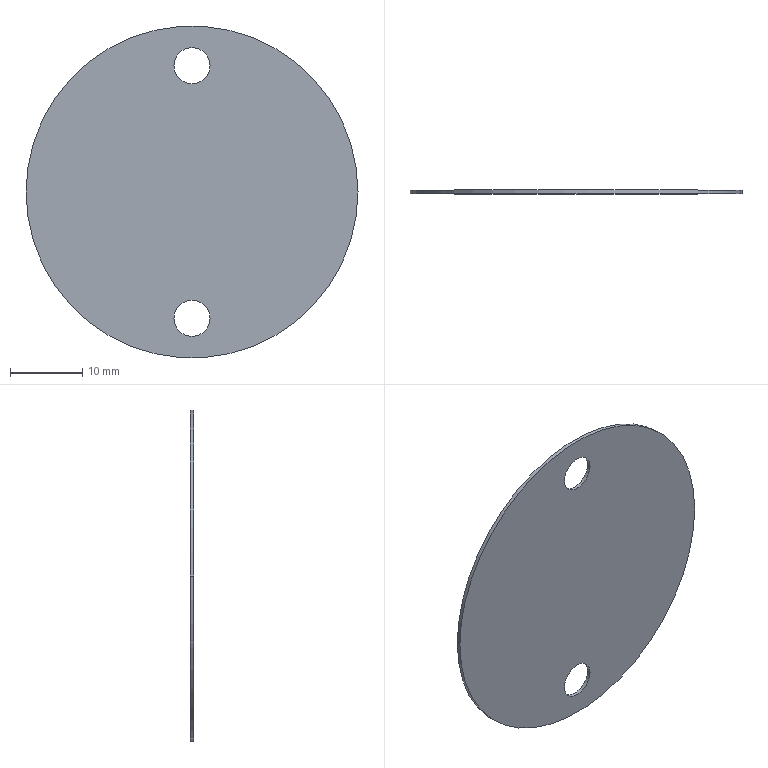Part | STEP file | 1 solid | 8 faces | box 46 x 0.5 x 46 mm | volume 811.316 mm3 | cylinder 6 | plane 2 | commonest cylinder face diameters 5 x4 46 x2
STEP:
#1=CARTESIAN_POINT('',(0.,0.,0.));
#2=DIRECTION('',(0.,0.,1.));
#3=DIRECTION('',(1.,0.,0.));
#4=AXIS2_PLACEMENT_3D('',#1,#2,#3);
#5=CARTESIAN_POINT('',(-2.5,-96.5,17.5));
#6=VERTEX_POINT('',#5);
#7=CARTESIAN_POINT('',(-2.5,-96.,17.5));
#8=VERTEX_POINT('',#7);
#9=CARTESIAN_POINT('',(-2.5,-96.5,17.5));
#10=DIRECTION('',(0.,1.,0.));
#11=VECTOR('',#10,1.);
#12=LINE('',#9,#11);
#13=CARTESIAN_POINT('',(0.,-96.5,17.5));
#14=DIRECTION('',(0.,1.,0.));
#15=DIRECTION('',(-1.,0.,0.));
#16=AXIS2_PLACEMENT_3D('',#13,#14,#15);
#17=CYLINDRICAL_SURFACE('',#16,2.5);
#18=CARTESIAN_POINT('',(6.283,0.));
#19=DIRECTION('',(0.,1.));
#20=VECTOR('',#19,1.);
#21=LINE('',#18,#20);
#22=(GEOMETRIC_REPRESENTATION_CONTEXT(2)PARAMETRIC_REPRESENTATION_CONTEXT()REPRESENTATION_CONTEXT('',''));
#23=DEFINITIONAL_REPRESENTATION('',(#21),#22);
#24=PCURVE('',#17,#23);
#25=CARTESIAN_POINT('',(0.,-96.5,17.5));
#26=DIRECTION('',(0.,1.,0.));
#27=DIRECTION('',(-1.,0.,0.));
#28=AXIS2_PLACEMENT_3D('',#25,#26,#27);
#29=CYLINDRICAL_SURFACE('',#28,2.5);
#30=CARTESIAN_POINT('',(0.,0.));
#31=DIRECTION('',(0.,1.));
#32=VECTOR('',#31,1.);
#33=LINE('',#30,#32);
#34=(GEOMETRIC_REPRESENTATION_CONTEXT(2)PARAMETRIC_REPRESENTATION_CONTEXT()REPRESENTATION_CONTEXT('',''));
#35=DEFINITIONAL_REPRESENTATION('',(#33),#34);
#36=PCURVE('',#29,#35);
#37=SURFACE_CURVE('',#12,(#24,#36),.PCURVE_S1.);
#38=EDGE_CURVE('',#6,#8,#37,.T.);
#39=ORIENTED_EDGE('',*,*,#38,.T.);
#40=CARTESIAN_POINT('',(2.5,-96.,17.5));
#41=VERTEX_POINT('',#40);
#42=CARTESIAN_POINT('',(0.,-96.,17.5));
#43=DIRECTION('',(0.,1.,0.));
#44=DIRECTION('',(-1.,0.,0.));
#45=AXIS2_PLACEMENT_3D('',#42,#43,#44);
#46=CIRCLE('',#45,2.5);
#47=CARTESIAN_POINT('',(0.,0.5));
#48=DIRECTION('',(1.,0.));
#49=VECTOR('',#48,1.);
#50=LINE('',#47,#49);
#51=(GEOMETRIC_REPRESENTATION_CONTEXT(2)PARAMETRIC_REPRESENTATION_CONTEXT()REPRESENTATION_CONTEXT('',''));
#52=DEFINITIONAL_REPRESENTATION('',(#50),#51);
#53=PCURVE('',#17,#52);
#54=CARTESIAN_POINT('',(23.92,-96.,23.92));
#55=DIRECTION('',(0.,1.,0.));
#56=DIRECTION('',(0.,0.,-1.));
#57=AXIS2_PLACEMENT_3D('',#54,#55,#56);
#58=PLANE('',#57);
#59=CARTESIAN_POINT('',(6.42,23.92));
#60=DIRECTION('',(0.,1.));
#61=AXIS2_PLACEMENT_2D('',#59,#60);
#62=CIRCLE('',#61,2.5);
#63=(GEOMETRIC_REPRESENTATION_CONTEXT(2)PARAMETRIC_REPRESENTATION_CONTEXT()REPRESENTATION_CONTEXT('',''));
#64=DEFINITIONAL_REPRESENTATION('',(#62),#63);
#65=PCURVE('',#58,#64);
#66=SURFACE_CURVE('',#46,(#53,#65),.PCURVE_S1.);
#67=EDGE_CURVE('',#41,#8,#66,.T.);
#68=ORIENTED_EDGE('',*,*,#67,.F.);
#69=CARTESIAN_POINT('',(2.5,-96.5,17.5));
#70=VERTEX_POINT('',#69);
#71=CARTESIAN_POINT('',(2.5,-96.5,17.5));
#72=DIRECTION('',(0.,1.,0.));
#73=VECTOR('',#72,1.);
#74=LINE('',#71,#73);
#75=CARTESIAN_POINT('',(3.142,0.));
#76=DIRECTION('',(0.,1.));
#77=VECTOR('',#76,1.);
#78=LINE('',#75,#77);
#79=(GEOMETRIC_REPRESENTATION_CONTEXT(2)PARAMETRIC_REPRESENTATION_CONTEXT()REPRESENTATION_CONTEXT('',''));
#80=DEFINITIONAL_REPRESENTATION('',(#78),#79);
#81=PCURVE('',#17,#80);
#82=CARTESIAN_POINT('',(3.142,0.));
#83=DIRECTION('',(0.,1.));
#84=VECTOR('',#83,1.);
#85=LINE('',#82,#84);
#86=(GEOMETRIC_REPRESENTATION_CONTEXT(2)PARAMETRIC_REPRESENTATION_CONTEXT()REPRESENTATION_CONTEXT('',''));
#87=DEFINITIONAL_REPRESENTATION('',(#85),#86);
#88=PCURVE('',#29,#87);
#89=SURFACE_CURVE('',#74,(#81,#88),.PCURVE_S1.);
#90=EDGE_CURVE('',#70,#41,#89,.T.);
#91=ORIENTED_EDGE('',*,*,#90,.F.);
#92=CARTESIAN_POINT('',(0.,-96.5,17.5));
#93=DIRECTION('',(0.,-1.,0.));
#94=DIRECTION('',(-1.,0.,0.));
#95=AXIS2_PLACEMENT_3D('',#92,#93,#94);
#96=CIRCLE('',#95,2.5);
#97=CARTESIAN_POINT('',(6.283,0.));
#98=DIRECTION('',(-1.,0.));
#99=VECTOR('',#98,1.);
#100=LINE('',#97,#99);
#101=(GEOMETRIC_REPRESENTATION_CONTEXT(2)PARAMETRIC_REPRESENTATION_CONTEXT()REPRESENTATION_CONTEXT('',''));
#102=DEFINITIONAL_REPRESENTATION('',(#100),#101);
#103=PCURVE('',#17,#102);
#104=CARTESIAN_POINT('',(23.92,-96.5,23.92));
#105=DIRECTION('',(0.,1.,0.));
#106=DIRECTION('',(0.,0.,-1.));
#107=AXIS2_PLACEMENT_3D('',#104,#105,#106);
#108=PLANE('',#107);
#109=CARTESIAN_POINT('',(6.42,26.42));
#110=CARTESIAN_POINT('',(10.75,26.42));
#111=CARTESIAN_POINT('',(8.585,22.67));
#112=CARTESIAN_POINT('',(6.42,18.92));
#113=CARTESIAN_POINT('',(4.255,22.67));
#114=CARTESIAN_POINT('',(2.09,26.42));
#115=CARTESIAN_POINT('',(6.42,26.42));
#116=(BOUNDED_CURVE()B_SPLINE_CURVE(2,(#109,#110,#111,#112,#113,#114,#115),.UNSPECIFIED.,.T.,.F.)B_SPLINE_CURVE_WITH_KNOTS((1,2,2,2,2,1),(-2.094,0.,2.094,4.189,6.283,8.378),.UNSPECIFIED.)CURVE()GEOMETRIC_REPRESENTATION_ITEM()RATIONAL_B_SPLINE_CURVE((1.,0.5,1.,0.5,1.,0.5,1.))REPRESENTATION_ITEM(''));
#117=(GEOMETRIC_REPRESENTATION_CONTEXT(2)PARAMETRIC_REPRESENTATION_CONTEXT()REPRESENTATION_CONTEXT('',''));
#118=DEFINITIONAL_REPRESENTATION('',(#116),#117);
#119=PCURVE('',#108,#118);
#120=SURFACE_CURVE('',#96,(#103,#119),.PCURVE_S1.);
#121=EDGE_CURVE('',#6,#70,#120,.T.);
#122=ORIENTED_EDGE('',*,*,#121,.F.);
#123=EDGE_LOOP('',(#39,#68,#91,#122));
#124=FACE_BOUND('',#123,.F.);
#125=ADVANCED_FACE('',(#124),#17,.F.);
#126=CARTESIAN_POINT('',(-2.5,-96.5,-17.5));
#127=VERTEX_POINT('',#126);
#128=CARTESIAN_POINT('',(-2.5,-96.,-17.5));
#129=VERTEX_POINT('',#128);
#130=CARTESIAN_POINT('',(-2.5,-96.5,-17.5));
#131=DIRECTION('',(0.,1.,0.));
#132=VECTOR('',#131,1.);
#133=LINE('',#130,#132);
#134=CARTESIAN_POINT('',(0.,-96.5,-17.5));
#135=DIRECTION('',(0.,1.,0.));
#136=DIRECTION('',(-1.,0.,0.));
#137=AXIS2_PLACEMENT_3D('',#134,#135,#136);
#138=CYLINDRICAL_SURFACE('',#137,2.5);
#139=CARTESIAN_POINT('',(6.283,0.));
#140=DIRECTION('',(0.,1.));
#141=VECTOR('',#140,1.);
#142=LINE('',#139,#141);
#143=(GEOMETRIC_REPRESENTATION_CONTEXT(2)PARAMETRIC_REPRESENTATION_CONTEXT()REPRESENTATION_CONTEXT('',''));
#144=DEFINITIONAL_REPRESENTATION('',(#142),#143);
#145=PCURVE('',#138,#144);
#146=CARTESIAN_POINT('',(0.,-96.5,-17.5));
#147=DIRECTION('',(0.,1.,0.));
#148=DIRECTION('',(-1.,0.,0.));
#149=AXIS2_PLACEMENT_3D('',#146,#147,#148);
#150=CYLINDRICAL_SURFACE('',#149,2.5);
#151=CARTESIAN_POINT('',(0.,0.));
#152=DIRECTION('',(0.,1.));
#153=VECTOR('',#152,1.);
#154=LINE('',#151,#153);
#155=(GEOMETRIC_REPRESENTATION_CONTEXT(2)PARAMETRIC_REPRESENTATION_CONTEXT()REPRESENTATION_CONTEXT('',''));
#156=DEFINITIONAL_REPRESENTATION('',(#154),#155);
#157=PCURVE('',#150,#156);
#158=SURFACE_CURVE('',#133,(#145,#157),.PCURVE_S1.);
#159=EDGE_CURVE('',#127,#129,#158,.T.);
#160=ORIENTED_EDGE('',*,*,#159,.T.);
#161=CARTESIAN_POINT('',(2.5,-96.,-17.5));
#162=VERTEX_POINT('',#161);
#163=CARTESIAN_POINT('',(0.,-96.,-17.5));
#164=DIRECTION('',(0.,1.,0.));
#165=DIRECTION('',(-1.,0.,0.));
#166=AXIS2_PLACEMENT_3D('',#163,#164,#165);
#167=CIRCLE('',#166,2.5);
#168=CARTESIAN_POINT('',(0.,0.5));
#169=DIRECTION('',(1.,0.));
#170=VECTOR('',#169,1.);
#171=LINE('',#168,#170);
#172=(GEOMETRIC_REPRESENTATION_CONTEXT(2)PARAMETRIC_REPRESENTATION_CONTEXT()REPRESENTATION_CONTEXT('',''));
#173=DEFINITIONAL_REPRESENTATION('',(#171),#172);
#174=PCURVE('',#138,#173);
#175=CARTESIAN_POINT('',(41.42,23.92));
#176=DIRECTION('',(0.,1.));
#177=AXIS2_PLACEMENT_2D('',#175,#176);
#178=CIRCLE('',#177,2.5);
#179=(GEOMETRIC_REPRESENTATION_CONTEXT(2)PARAMETRIC_REPRESENTATION_CONTEXT()REPRESENTATION_CONTEXT('',''));
#180=DEFINITIONAL_REPRESENTATION('',(#178),#179);
#181=PCURVE('',#58,#180);
#182=SURFACE_CURVE('',#167,(#174,#181),.PCURVE_S1.);
#183=EDGE_CURVE('',#162,#129,#182,.T.);
#184=ORIENTED_EDGE('',*,*,#183,.F.);
#185=CARTESIAN_POINT('',(2.5,-96.5,-17.5));
#186=VERTEX_POINT('',#185);
#187=CARTESIAN_POINT('',(2.5,-96.5,-17.5));
#188=DIRECTION('',(0.,1.,0.));
#189=VECTOR('',#188,1.);
#190=LINE('',#187,#189);
#191=CARTESIAN_POINT('',(3.142,0.));
#192=DIRECTION('',(0.,1.));
#193=VECTOR('',#192,1.);
#194=LINE('',#191,#193);
#195=(GEOMETRIC_REPRESENTATION_CONTEXT(2)PARAMETRIC_REPRESENTATION_CONTEXT()REPRESENTATION_CONTEXT('',''));
#196=DEFINITIONAL_REPRESENTATION('',(#194),#195);
#197=PCURVE('',#138,#196);
#198=CARTESIAN_POINT('',(3.142,0.));
#199=DIRECTION('',(0.,1.));
#200=VECTOR('',#199,1.);
#201=LINE('',#198,#200);
#202=(GEOMETRIC_REPRESENTATION_CONTEXT(2)PARAMETRIC_REPRESENTATION_CONTEXT()REPRESENTATION_CONTEXT('',''));
#203=DEFINITIONAL_REPRESENTATION('',(#201),#202);
#204=PCURVE('',#150,#203);
#205=SURFACE_CURVE('',#190,(#197,#204),.PCURVE_S1.);
#206=EDGE_CURVE('',#186,#162,#205,.T.);
#207=ORIENTED_EDGE('',*,*,#206,.F.);
#208=CARTESIAN_POINT('',(0.,-96.5,-17.5));
#209=DIRECTION('',(0.,-1.,0.));
#210=DIRECTION('',(-1.,0.,0.));
#211=AXIS2_PLACEMENT_3D('',#208,#209,#210);
#212=CIRCLE('',#211,2.5);
#213=CARTESIAN_POINT('',(6.283,0.));
#214=DIRECTION('',(-1.,0.));
#215=VECTOR('',#214,1.);
#216=LINE('',#213,#215);
#217=(GEOMETRIC_REPRESENTATION_CONTEXT(2)PARAMETRIC_REPRESENTATION_CONTEXT()REPRESENTATION_CONTEXT('',''));
#218=DEFINITIONAL_REPRESENTATION('',(#216),#217);
#219=PCURVE('',#138,#218);
#220=CARTESIAN_POINT('',(41.42,26.42));
#221=CARTESIAN_POINT('',(45.75,26.42));
#222=CARTESIAN_POINT('',(43.585,22.67));
#223=CARTESIAN_POINT('',(41.42,18.92));
#224=CARTESIAN_POINT('',(39.255,22.67));
#225=CARTESIAN_POINT('',(37.09,26.42));
#226=CARTESIAN_POINT('',(41.42,26.42));
#227=(BOUNDED_CURVE()B_SPLINE_CURVE(2,(#220,#221,#222,#223,#224,#225,#226),.UNSPECIFIED.,.T.,.F.)B_SPLINE_CURVE_WITH_KNOTS((1,2,2,2,2,1),(-2.094,0.,2.094,4.189,6.283,8.378),.UNSPECIFIED.)CURVE()GEOMETRIC_REPRESENTATION_ITEM()RATIONAL_B_SPLINE_CURVE((1.,0.5,1.,0.5,1.,0.5,1.))REPRESENTATION_ITEM(''));
#228=(GEOMETRIC_REPRESENTATION_CONTEXT(2)PARAMETRIC_REPRESENTATION_CONTEXT()REPRESENTATION_CONTEXT('',''));
#229=DEFINITIONAL_REPRESENTATION('',(#227),#228);
#230=PCURVE('',#108,#229);
#231=SURFACE_CURVE('',#212,(#219,#230),.PCURVE_S1.);
#232=EDGE_CURVE('',#127,#186,#231,.T.);
#233=ORIENTED_EDGE('',*,*,#232,.F.);
#234=EDGE_LOOP('',(#160,#184,#207,#233));
#235=FACE_BOUND('',#234,.F.);
#236=ADVANCED_FACE('',(#235),#138,.F.);
#237=CARTESIAN_POINT('',(-23.,-96.5,0.));
#238=VERTEX_POINT('',#237);
#239=CARTESIAN_POINT('',(23.,-96.5,0.));
#240=VERTEX_POINT('',#239);
#241=CARTESIAN_POINT('',(0.,-96.5,0.));
#242=DIRECTION('',(0.,1.,0.));
#243=DIRECTION('',(-1.,0.,0.));
#244=AXIS2_PLACEMENT_3D('',#241,#242,#243);
#245=CIRCLE('',#244,23.);
#246=CARTESIAN_POINT('',(0.,-96.5,0.));
#247=DIRECTION('',(0.,1.,0.));
#248=DIRECTION('',(-1.,0.,0.));
#249=AXIS2_PLACEMENT_3D('',#246,#247,#248);
#250=CYLINDRICAL_SURFACE('',#249,23.);
#251=CARTESIAN_POINT('',(0.,0.));
#252=DIRECTION('',(1.,0.));
#253=VECTOR('',#252,1.);
#254=LINE('',#251,#253);
#255=(GEOMETRIC_REPRESENTATION_CONTEXT(2)PARAMETRIC_REPRESENTATION_CONTEXT()REPRESENTATION_CONTEXT('',''));
#256=DEFINITIONAL_REPRESENTATION('',(#254),#255);
#257=PCURVE('',#250,#256);
#258=CARTESIAN_POINT('',(23.92,23.92));
#259=DIRECTION('',(0.,1.));
#260=AXIS2_PLACEMENT_2D('',#258,#259);
#261=CIRCLE('',#260,23.);
#262=(GEOMETRIC_REPRESENTATION_CONTEXT(2)PARAMETRIC_REPRESENTATION_CONTEXT()REPRESENTATION_CONTEXT('',''));
#263=DEFINITIONAL_REPRESENTATION('',(#261),#262);
#264=PCURVE('',#108,#263);
#265=SURFACE_CURVE('',#245,(#257,#264),.PCURVE_S1.);
#266=EDGE_CURVE('',#238,#240,#265,.T.);
#267=ORIENTED_EDGE('',*,*,#266,.T.);
#268=CARTESIAN_POINT('',(23.,-96.,0.));
#269=VERTEX_POINT('',#268);
#270=CARTESIAN_POINT('',(23.,-96.5,0.));
#271=DIRECTION('',(0.,1.,0.));
#272=VECTOR('',#271,1.);
#273=LINE('',#270,#272);
#274=CARTESIAN_POINT('',(3.142,0.));
#275=DIRECTION('',(0.,1.));
#276=VECTOR('',#275,1.);
#277=LINE('',#274,#276);
#278=(GEOMETRIC_REPRESENTATION_CONTEXT(2)PARAMETRIC_REPRESENTATION_CONTEXT()REPRESENTATION_CONTEXT('',''));
#279=DEFINITIONAL_REPRESENTATION('',(#277),#278);
#280=PCURVE('',#250,#279);
#281=CARTESIAN_POINT('',(0.,-96.5,0.));
#282=DIRECTION('',(0.,1.,0.));
#283=DIRECTION('',(-1.,0.,0.));
#284=AXIS2_PLACEMENT_3D('',#281,#282,#283);
#285=CYLINDRICAL_SURFACE('',#284,23.);
#286=CARTESIAN_POINT('',(3.142,0.));
#287=DIRECTION('',(0.,1.));
#288=VECTOR('',#287,1.);
#289=LINE('',#286,#288);
#290=(GEOMETRIC_REPRESENTATION_CONTEXT(2)PARAMETRIC_REPRESENTATION_CONTEXT()REPRESENTATION_CONTEXT('',''));
#291=DEFINITIONAL_REPRESENTATION('',(#289),#290);
#292=PCURVE('',#285,#291);
#293=SURFACE_CURVE('',#273,(#280,#292),.PCURVE_S1.);
#294=EDGE_CURVE('',#240,#269,#293,.T.);
#295=ORIENTED_EDGE('',*,*,#294,.T.);
#296=CARTESIAN_POINT('',(-23.,-96.,0.));
#297=VERTEX_POINT('',#296);
#298=CARTESIAN_POINT('',(0.,-96.,0.));
#299=DIRECTION('',(0.,1.,0.));
#300=DIRECTION('',(-1.,0.,0.));
#301=AXIS2_PLACEMENT_3D('',#298,#299,#300);
#302=CIRCLE('',#301,23.);
#303=CARTESIAN_POINT('',(0.,0.5));
#304=DIRECTION('',(1.,0.));
#305=VECTOR('',#304,1.);
#306=LINE('',#303,#305);
#307=(GEOMETRIC_REPRESENTATION_CONTEXT(2)PARAMETRIC_REPRESENTATION_CONTEXT()REPRESENTATION_CONTEXT('',''));
#308=DEFINITIONAL_REPRESENTATION('',(#306),#307);
#309=PCURVE('',#250,#308);
#310=CARTESIAN_POINT('',(23.92,23.92));
#311=DIRECTION('',(0.,1.));
#312=AXIS2_PLACEMENT_2D('',#310,#311);
#313=CIRCLE('',#312,23.);
#314=(GEOMETRIC_REPRESENTATION_CONTEXT(2)PARAMETRIC_REPRESENTATION_CONTEXT()REPRESENTATION_CONTEXT('',''));
#315=DEFINITIONAL_REPRESENTATION('',(#313),#314);
#316=PCURVE('',#58,#315);
#317=SURFACE_CURVE('',#302,(#309,#316),.PCURVE_S1.);
#318=EDGE_CURVE('',#297,#269,#317,.T.);
#319=ORIENTED_EDGE('',*,*,#318,.F.);
#320=CARTESIAN_POINT('',(-23.,-96.5,0.));
#321=DIRECTION('',(0.,1.,0.));
#322=VECTOR('',#321,1.);
#323=LINE('',#320,#322);
#324=CARTESIAN_POINT('',(0.,0.));
#325=DIRECTION('',(0.,1.));
#326=VECTOR('',#325,1.);
#327=LINE('',#324,#326);
#328=(GEOMETRIC_REPRESENTATION_CONTEXT(2)PARAMETRIC_REPRESENTATION_CONTEXT()REPRESENTATION_CONTEXT('',''));
#329=DEFINITIONAL_REPRESENTATION('',(#327),#328);
#330=PCURVE('',#250,#329);
#331=CARTESIAN_POINT('',(6.283,0.));
#332=DIRECTION('',(0.,1.));
#333=VECTOR('',#332,1.);
#334=LINE('',#331,#333);
#335=(GEOMETRIC_REPRESENTATION_CONTEXT(2)PARAMETRIC_REPRESENTATION_CONTEXT()REPRESENTATION_CONTEXT('',''));
#336=DEFINITIONAL_REPRESENTATION('',(#334),#335);
#337=PCURVE('',#285,#336);
#338=SURFACE_CURVE('',#323,(#330,#337),.PCURVE_S1.);
#339=EDGE_CURVE('',#238,#297,#338,.T.);
#340=ORIENTED_EDGE('',*,*,#339,.F.);
#341=EDGE_LOOP('',(#267,#295,#319,#340));
#342=FACE_BOUND('',#341,.T.);
#343=ADVANCED_FACE('',(#342),#250,.T.);
#344=CARTESIAN_POINT('',(0.,-96.,17.5));
#345=DIRECTION('',(0.,1.,0.));
#346=DIRECTION('',(-1.,0.,0.));
#347=AXIS2_PLACEMENT_3D('',#344,#345,#346);
#348=CIRCLE('',#347,2.5);
#349=CARTESIAN_POINT('',(6.42,23.92));
#350=DIRECTION('',(0.,1.));
#351=AXIS2_PLACEMENT_2D('',#349,#350);
#352=CIRCLE('',#351,2.5);
#353=(GEOMETRIC_REPRESENTATION_CONTEXT(2)PARAMETRIC_REPRESENTATION_CONTEXT()REPRESENTATION_CONTEXT('',''));
#354=DEFINITIONAL_REPRESENTATION('',(#352),#353);
#355=PCURVE('',#58,#354);
#356=CARTESIAN_POINT('',(0.,0.5));
#357=DIRECTION('',(1.,0.));
#358=VECTOR('',#357,1.);
#359=LINE('',#356,#358);
#360=(GEOMETRIC_REPRESENTATION_CONTEXT(2)PARAMETRIC_REPRESENTATION_CONTEXT()REPRESENTATION_CONTEXT('',''));
#361=DEFINITIONAL_REPRESENTATION('',(#359),#360);
#362=PCURVE('',#29,#361);
#363=SURFACE_CURVE('',#348,(#355,#362),.PCURVE_S1.);
#364=EDGE_CURVE('',#8,#41,#363,.T.);
#365=ORIENTED_EDGE('',*,*,#364,.F.);
#366=ORIENTED_EDGE('',*,*,#67,.F.);
#367=EDGE_LOOP('',(#365,#366));
#368=FACE_BOUND('',#367,.T.);
#369=CARTESIAN_POINT('',(0.,-96.,-17.5));
#370=DIRECTION('',(0.,1.,0.));
#371=DIRECTION('',(-1.,0.,0.));
#372=AXIS2_PLACEMENT_3D('',#369,#370,#371);
#373=CIRCLE('',#372,2.5);
#374=CARTESIAN_POINT('',(41.42,23.92));
#375=DIRECTION('',(0.,1.));
#376=AXIS2_PLACEMENT_2D('',#374,#375);
#377=CIRCLE('',#376,2.5);
#378=(GEOMETRIC_REPRESENTATION_CONTEXT(2)PARAMETRIC_REPRESENTATION_CONTEXT()REPRESENTATION_CONTEXT('',''));
#379=DEFINITIONAL_REPRESENTATION('',(#377),#378);
#380=PCURVE('',#58,#379);
#381=CARTESIAN_POINT('',(0.,0.5));
#382=DIRECTION('',(1.,0.));
#383=VECTOR('',#382,1.);
#384=LINE('',#381,#383);
#385=(GEOMETRIC_REPRESENTATION_CONTEXT(2)PARAMETRIC_REPRESENTATION_CONTEXT()REPRESENTATION_CONTEXT('',''));
#386=DEFINITIONAL_REPRESENTATION('',(#384),#385);
#387=PCURVE('',#150,#386);
#388=SURFACE_CURVE('',#373,(#380,#387),.PCURVE_S1.);
#389=EDGE_CURVE('',#129,#162,#388,.T.);
#390=ORIENTED_EDGE('',*,*,#389,.F.);
#391=ORIENTED_EDGE('',*,*,#183,.F.);
#392=EDGE_LOOP('',(#390,#391));
#393=FACE_BOUND('',#392,.T.);
#394=ORIENTED_EDGE('',*,*,#318,.T.);
#395=CARTESIAN_POINT('',(0.,-96.,0.));
#396=DIRECTION('',(0.,1.,0.));
#397=DIRECTION('',(-1.,0.,0.));
#398=AXIS2_PLACEMENT_3D('',#395,#396,#397);
#399=CIRCLE('',#398,23.);
#400=CARTESIAN_POINT('',(23.92,23.92));
#401=DIRECTION('',(0.,1.));
#402=AXIS2_PLACEMENT_2D('',#400,#401);
#403=CIRCLE('',#402,23.);
#404=(GEOMETRIC_REPRESENTATION_CONTEXT(2)PARAMETRIC_REPRESENTATION_CONTEXT()REPRESENTATION_CONTEXT('',''));
#405=DEFINITIONAL_REPRESENTATION('',(#403),#404);
#406=PCURVE('',#58,#405);
#407=CARTESIAN_POINT('',(0.,0.5));
#408=DIRECTION('',(1.,0.));
#409=VECTOR('',#408,1.);
#410=LINE('',#407,#409);
#411=(GEOMETRIC_REPRESENTATION_CONTEXT(2)PARAMETRIC_REPRESENTATION_CONTEXT()REPRESENTATION_CONTEXT('',''));
#412=DEFINITIONAL_REPRESENTATION('',(#410),#411);
#413=PCURVE('',#285,#412);
#414=SURFACE_CURVE('',#399,(#406,#413),.PCURVE_S1.);
#415=EDGE_CURVE('',#269,#297,#414,.T.);
#416=ORIENTED_EDGE('',*,*,#415,.T.);
#417=EDGE_LOOP('',(#394,#416));
#418=FACE_BOUND('',#417,.T.);
#419=ADVANCED_FACE('',(#368,#393,#418),#58,.T.);
#420=ORIENTED_EDGE('',*,*,#294,.F.);
#421=CARTESIAN_POINT('',(0.,-96.5,0.));
#422=DIRECTION('',(0.,1.,0.));
#423=DIRECTION('',(-1.,0.,0.));
#424=AXIS2_PLACEMENT_3D('',#421,#422,#423);
#425=CIRCLE('',#424,23.);
#426=CARTESIAN_POINT('',(0.,0.));
#427=DIRECTION('',(1.,0.));
#428=VECTOR('',#427,1.);
#429=LINE('',#426,#428);
#430=(GEOMETRIC_REPRESENTATION_CONTEXT(2)PARAMETRIC_REPRESENTATION_CONTEXT()REPRESENTATION_CONTEXT('',''));
#431=DEFINITIONAL_REPRESENTATION('',(#429),#430);
#432=PCURVE('',#285,#431);
#433=CARTESIAN_POINT('',(23.92,23.92));
#434=DIRECTION('',(0.,1.));
#435=AXIS2_PLACEMENT_2D('',#433,#434);
#436=CIRCLE('',#435,23.);
#437=(GEOMETRIC_REPRESENTATION_CONTEXT(2)PARAMETRIC_REPRESENTATION_CONTEXT()REPRESENTATION_CONTEXT('',''));
#438=DEFINITIONAL_REPRESENTATION('',(#436),#437);
#439=PCURVE('',#108,#438);
#440=SURFACE_CURVE('',#425,(#432,#439),.PCURVE_S1.);
#441=EDGE_CURVE('',#240,#238,#440,.T.);
#442=ORIENTED_EDGE('',*,*,#441,.T.);
#443=ORIENTED_EDGE('',*,*,#339,.T.);
#444=ORIENTED_EDGE('',*,*,#415,.F.);
#445=EDGE_LOOP('',(#420,#442,#443,#444));
#446=FACE_BOUND('',#445,.T.);
#447=ADVANCED_FACE('',(#446),#285,.T.);
#448=ORIENTED_EDGE('',*,*,#389,.F.);
#449=ORIENTED_EDGE('',*,*,#159,.F.);
#450=CARTESIAN_POINT('',(0.,-96.5,-17.5));
#451=DIRECTION('',(0.,-1.,0.));
#452=DIRECTION('',(-1.,0.,0.));
#453=AXIS2_PLACEMENT_3D('',#450,#451,#452);
#454=CIRCLE('',#453,2.5);
#455=CARTESIAN_POINT('',(6.283,0.));
#456=DIRECTION('',(-1.,0.));
#457=VECTOR('',#456,1.);
#458=LINE('',#455,#457);
#459=(GEOMETRIC_REPRESENTATION_CONTEXT(2)PARAMETRIC_REPRESENTATION_CONTEXT()REPRESENTATION_CONTEXT('',''));
#460=DEFINITIONAL_REPRESENTATION('',(#458),#459);
#461=PCURVE('',#150,#460);
#462=CARTESIAN_POINT('',(41.42,26.42));
#463=CARTESIAN_POINT('',(45.75,26.42));
#464=CARTESIAN_POINT('',(43.585,22.67));
#465=CARTESIAN_POINT('',(41.42,18.92));
#466=CARTESIAN_POINT('',(39.255,22.67));
#467=CARTESIAN_POINT('',(37.09,26.42));
#468=CARTESIAN_POINT('',(41.42,26.42));
#469=(BOUNDED_CURVE()B_SPLINE_CURVE(2,(#462,#463,#464,#465,#466,#467,#468),.UNSPECIFIED.,.T.,.F.)B_SPLINE_CURVE_WITH_KNOTS((1,2,2,2,2,1),(-2.094,0.,2.094,4.189,6.283,8.378),.UNSPECIFIED.)CURVE()GEOMETRIC_REPRESENTATION_ITEM()RATIONAL_B_SPLINE_CURVE((1.,0.5,1.,0.5,1.,0.5,1.))REPRESENTATION_ITEM(''));
#470=(GEOMETRIC_REPRESENTATION_CONTEXT(2)PARAMETRIC_REPRESENTATION_CONTEXT()REPRESENTATION_CONTEXT('',''));
#471=DEFINITIONAL_REPRESENTATION('',(#469),#470);
#472=PCURVE('',#108,#471);
#473=SURFACE_CURVE('',#454,(#461,#472),.PCURVE_S1.);
#474=EDGE_CURVE('',#186,#127,#473,.T.);
#475=ORIENTED_EDGE('',*,*,#474,.F.);
#476=ORIENTED_EDGE('',*,*,#206,.T.);
#477=EDGE_LOOP('',(#448,#449,#475,#476));
#478=FACE_BOUND('',#477,.F.);
#479=ADVANCED_FACE('',(#478),#150,.F.);
#480=ORIENTED_EDGE('',*,*,#364,.F.);
#481=ORIENTED_EDGE('',*,*,#38,.F.);
#482=CARTESIAN_POINT('',(0.,-96.5,17.5));
#483=DIRECTION('',(0.,-1.,0.));
#484=DIRECTION('',(-1.,0.,0.));
#485=AXIS2_PLACEMENT_3D('',#482,#483,#484);
#486=CIRCLE('',#485,2.5);
#487=CARTESIAN_POINT('',(6.283,0.));
#488=DIRECTION('',(-1.,0.));
#489=VECTOR('',#488,1.);
#490=LINE('',#487,#489);
#491=(GEOMETRIC_REPRESENTATION_CONTEXT(2)PARAMETRIC_REPRESENTATION_CONTEXT()REPRESENTATION_CONTEXT('',''));
#492=DEFINITIONAL_REPRESENTATION('',(#490),#491);
#493=PCURVE('',#29,#492);
#494=CARTESIAN_POINT('',(6.42,26.42));
#495=CARTESIAN_POINT('',(10.75,26.42));
#496=CARTESIAN_POINT('',(8.585,22.67));
#497=CARTESIAN_POINT('',(6.42,18.92));
#498=CARTESIAN_POINT('',(4.255,22.67));
#499=CARTESIAN_POINT('',(2.09,26.42));
#500=CARTESIAN_POINT('',(6.42,26.42));
#501=(BOUNDED_CURVE()B_SPLINE_CURVE(2,(#494,#495,#496,#497,#498,#499,#500),.UNSPECIFIED.,.T.,.F.)B_SPLINE_CURVE_WITH_KNOTS((1,2,2,2,2,1),(-2.094,0.,2.094,4.189,6.283,8.378),.UNSPECIFIED.)CURVE()GEOMETRIC_REPRESENTATION_ITEM()RATIONAL_B_SPLINE_CURVE((1.,0.5,1.,0.5,1.,0.5,1.))REPRESENTATION_ITEM(''));
#502=(GEOMETRIC_REPRESENTATION_CONTEXT(2)PARAMETRIC_REPRESENTATION_CONTEXT()REPRESENTATION_CONTEXT('',''));
#503=DEFINITIONAL_REPRESENTATION('',(#501),#502);
#504=PCURVE('',#108,#503);
#505=SURFACE_CURVE('',#486,(#493,#504),.PCURVE_S1.);
#506=EDGE_CURVE('',#70,#6,#505,.T.);
#507=ORIENTED_EDGE('',*,*,#506,.F.);
#508=ORIENTED_EDGE('',*,*,#90,.T.);
#509=EDGE_LOOP('',(#480,#481,#507,#508));
#510=FACE_BOUND('',#509,.F.);
#511=ADVANCED_FACE('',(#510),#29,.F.);
#512=ORIENTED_EDGE('',*,*,#121,.F.);
#513=ORIENTED_EDGE('',*,*,#506,.F.);
#514=EDGE_LOOP('',(#512,#513));
#515=FACE_BOUND('',#514,.T.);
#516=ORIENTED_EDGE('',*,*,#232,.F.);
#517=ORIENTED_EDGE('',*,*,#474,.F.);
#518=EDGE_LOOP('',(#516,#517));
#519=FACE_BOUND('',#518,.T.);
#520=ORIENTED_EDGE('',*,*,#266,.F.);
#521=ORIENTED_EDGE('',*,*,#441,.F.);
#522=EDGE_LOOP('',(#520,#521));
#523=FACE_BOUND('',#522,.T.);
#524=ADVANCED_FACE('',(#515,#519,#523),#108,.F.);
#525=CLOSED_SHELL('',(#125,#236,#343,#419,#447,#479,#511,#524));
#526=MANIFOLD_SOLID_BREP('',#525);
#527=(LENGTH_UNIT()NAMED_UNIT(*)SI_UNIT(.MILLI.,.METRE.));
#528=UNCERTAINTY_MEASURE_WITH_UNIT(LENGTH_MEASURE(0.0000001),#527,'','');
#529=(NAMED_UNIT(*)PLANE_ANGLE_UNIT()SI_UNIT($,.RADIAN.));
#530=(NAMED_UNIT(*)SI_UNIT($,.STERADIAN.)SOLID_ANGLE_UNIT());
#531=(GEOMETRIC_REPRESENTATION_CONTEXT(3)GLOBAL_UNCERTAINTY_ASSIGNED_CONTEXT((#528))GLOBAL_UNIT_ASSIGNED_CONTEXT((#527,#529,#530))REPRESENTATION_CONTEXT('',''));
#532=ADVANCED_BREP_SHAPE_REPRESENTATION('',(#4,#526),#531);